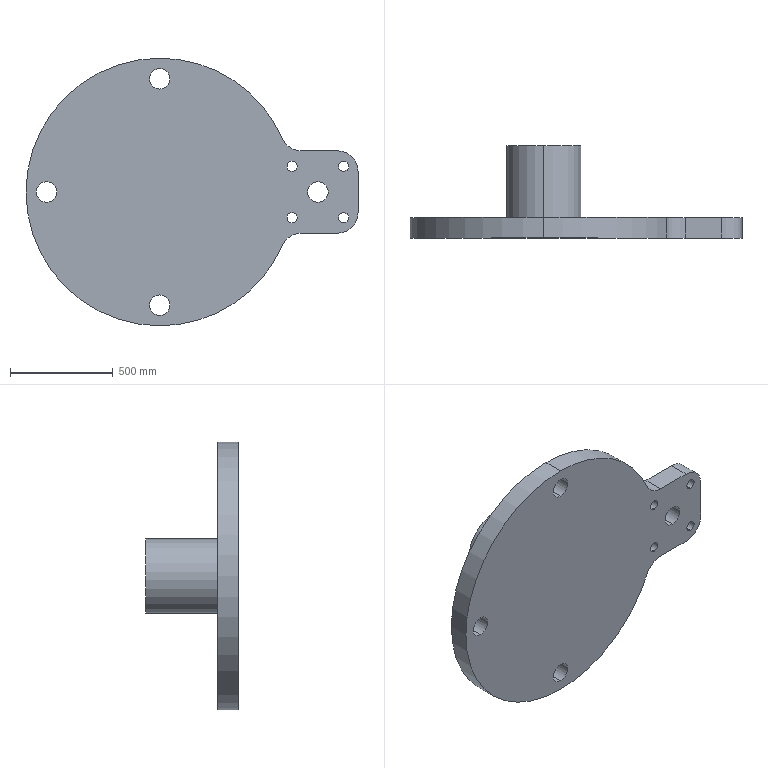Part | SolidWorks | features ICE 9, Extrusion 1, Fillet 1, MirrorPattern 1 | 1 solid | 31 faces | box 1613 x 450 x 1300 mm | volume 177120660 mm3 | cylinder 25 | plane 6 | commonest cylinder face diameters 50 x8 100 x8 200 x4 1300 x3 360 x2
STEP:
#1=CARTESIAN_POINT('',(768.466,750.,50.));
#2=VERTEX_POINT('',#1);
#3=CARTESIAN_POINT('',(768.466,750.,-50.));
#4=VERTEX_POINT('',#3);
#5=CARTESIAN_POINT('',(768.466,750.,0.));
#6=DIRECTION('',(0.,-1.,0.));
#7=DIRECTION('',(0.,0.,1.));
#8=AXIS2_PLACEMENT_3D('',#5,#6,#7);
#9=CIRCLE('',#8,50.);
#10=EDGE_CURVE('',#2,#4,#9,.T.);
#11=ORIENTED_EDGE('',*,*,#10,.T.);
#12=CARTESIAN_POINT('',(768.466,850.,-50.));
#13=VERTEX_POINT('',#12);
#14=CARTESIAN_POINT('',(768.466,-1050.001,-50.));
#15=DIRECTION('',(0.,1.,0.));
#16=VECTOR('',#15,1000.);
#17=LINE('',#14,#16);
#18=EDGE_CURVE('',#4,#13,#17,.T.);
#19=ORIENTED_EDGE('',*,*,#18,.T.);
#20=CARTESIAN_POINT('',(768.466,850.,50.));
#21=VERTEX_POINT('',#20);
#22=CARTESIAN_POINT('',(768.466,850.,0.));
#23=DIRECTION('',(0.,1.,0.));
#24=DIRECTION('',(0.,0.,1.));
#25=AXIS2_PLACEMENT_3D('',#22,#23,#24);
#26=CIRCLE('',#25,50.);
#27=EDGE_CURVE('',#13,#21,#26,.T.);
#28=ORIENTED_EDGE('',*,*,#27,.T.);
#29=CARTESIAN_POINT('',(768.466,-1050.001,50.));
#30=DIRECTION('',(0.,1.,0.));
#31=VECTOR('',#30,1000.);
#32=LINE('',#29,#31);
#33=EDGE_CURVE('',#2,#21,#32,.T.);
#34=ORIENTED_EDGE('',*,*,#33,.F.);
#35=EDGE_LOOP('',(#11,#19,#28,#34));
#36=FACE_OUTER_BOUND('',#35,.T.);
#37=CARTESIAN_POINT('',(768.466,-1050.001,0.));
#38=DIRECTION('',(0.,1.,0.));
#39=DIRECTION('',(0.,0.,1.));
#40=AXIS2_PLACEMENT_3D('',#37,#38,#39);
#41=CYLINDRICAL_SURFACE('',#40,50.);
#42=ADVANCED_FACE('',(#36),#41,.F.);
#43=CARTESIAN_POINT('',(893.466,750.,150.));
#44=VERTEX_POINT('',#43);
#45=CARTESIAN_POINT('',(893.466,750.,100.));
#46=VERTEX_POINT('',#45);
#47=CARTESIAN_POINT('',(893.466,750.,125.));
#48=DIRECTION('',(0.,-1.,0.));
#49=DIRECTION('',(0.,0.,1.));
#50=AXIS2_PLACEMENT_3D('',#47,#48,#49);
#51=CIRCLE('',#50,25.);
#52=EDGE_CURVE('',#44,#46,#51,.T.);
#53=ORIENTED_EDGE('',*,*,#52,.T.);
#54=CARTESIAN_POINT('',(893.466,850.,100.));
#55=VERTEX_POINT('',#54);
#56=CARTESIAN_POINT('',(893.466,-1050.001,100.));
#57=DIRECTION('',(0.,1.,0.));
#58=VECTOR('',#57,1000.);
#59=LINE('',#56,#58);
#60=EDGE_CURVE('',#46,#55,#59,.T.);
#61=ORIENTED_EDGE('',*,*,#60,.T.);
#62=CARTESIAN_POINT('',(893.466,850.,150.));
#63=VERTEX_POINT('',#62);
#64=CARTESIAN_POINT('',(893.466,850.,125.));
#65=DIRECTION('',(0.,1.,0.));
#66=DIRECTION('',(0.,0.,1.));
#67=AXIS2_PLACEMENT_3D('',#64,#65,#66);
#68=CIRCLE('',#67,25.);
#69=EDGE_CURVE('',#55,#63,#68,.T.);
#70=ORIENTED_EDGE('',*,*,#69,.T.);
#71=CARTESIAN_POINT('',(893.466,-1050.001,150.));
#72=DIRECTION('',(0.,1.,0.));
#73=VECTOR('',#72,1000.);
#74=LINE('',#71,#73);
#75=EDGE_CURVE('',#44,#63,#74,.T.);
#76=ORIENTED_EDGE('',*,*,#75,.F.);
#77=EDGE_LOOP('',(#53,#61,#70,#76));
#78=FACE_OUTER_BOUND('',#77,.T.);
#79=CARTESIAN_POINT('',(893.466,-1050.001,125.));
#80=DIRECTION('',(0.,1.,0.));
#81=DIRECTION('',(0.,0.,1.));
#82=AXIS2_PLACEMENT_3D('',#79,#80,#81);
#83=CYLINDRICAL_SURFACE('',#82,25.);
#84=ADVANCED_FACE('',(#78),#83,.F.);
#85=CARTESIAN_POINT('',(643.466,750.,150.));
#86=VERTEX_POINT('',#85);
#87=CARTESIAN_POINT('',(643.466,750.,100.));
#88=VERTEX_POINT('',#87);
#89=CARTESIAN_POINT('',(643.466,750.,125.));
#90=DIRECTION('',(0.,-1.,0.));
#91=DIRECTION('',(0.,0.,1.));
#92=AXIS2_PLACEMENT_3D('',#89,#90,#91);
#93=CIRCLE('',#92,25.);
#94=EDGE_CURVE('',#86,#88,#93,.T.);
#95=ORIENTED_EDGE('',*,*,#94,.T.);
#96=CARTESIAN_POINT('',(643.466,850.,100.));
#97=VERTEX_POINT('',#96);
#98=CARTESIAN_POINT('',(643.466,-1050.001,100.));
#99=DIRECTION('',(0.,1.,0.));
#100=VECTOR('',#99,1000.);
#101=LINE('',#98,#100);
#102=EDGE_CURVE('',#88,#97,#101,.T.);
#103=ORIENTED_EDGE('',*,*,#102,.T.);
#104=CARTESIAN_POINT('',(643.466,850.,150.));
#105=VERTEX_POINT('',#104);
#106=CARTESIAN_POINT('',(643.466,850.,125.));
#107=DIRECTION('',(0.,1.,0.));
#108=DIRECTION('',(0.,0.,1.));
#109=AXIS2_PLACEMENT_3D('',#106,#107,#108);
#110=CIRCLE('',#109,25.);
#111=EDGE_CURVE('',#97,#105,#110,.T.);
#112=ORIENTED_EDGE('',*,*,#111,.T.);
#113=CARTESIAN_POINT('',(643.466,-1050.001,150.));
#114=DIRECTION('',(0.,1.,0.));
#115=VECTOR('',#114,1000.);
#116=LINE('',#113,#115);
#117=EDGE_CURVE('',#86,#105,#116,.T.);
#118=ORIENTED_EDGE('',*,*,#117,.F.);
#119=EDGE_LOOP('',(#95,#103,#112,#118));
#120=FACE_OUTER_BOUND('',#119,.T.);
#121=CARTESIAN_POINT('',(643.466,-1050.001,125.));
#122=DIRECTION('',(0.,1.,0.));
#123=DIRECTION('',(0.,0.,1.));
#124=AXIS2_PLACEMENT_3D('',#121,#122,#123);
#125=CYLINDRICAL_SURFACE('',#124,25.);
#126=ADVANCED_FACE('',(#120),#125,.F.);
#127=CARTESIAN_POINT('',(643.466,750.,-100.));
#128=VERTEX_POINT('',#127);
#129=CARTESIAN_POINT('',(643.466,750.,-150.));
#130=VERTEX_POINT('',#129);
#131=CARTESIAN_POINT('',(643.466,750.,-125.));
#132=DIRECTION('',(0.,-1.,0.));
#133=DIRECTION('',(0.,0.,1.));
#134=AXIS2_PLACEMENT_3D('',#131,#132,#133);
#135=CIRCLE('',#134,25.);
#136=EDGE_CURVE('',#128,#130,#135,.T.);
#137=ORIENTED_EDGE('',*,*,#136,.T.);
#138=CARTESIAN_POINT('',(643.466,850.,-150.));
#139=VERTEX_POINT('',#138);
#140=CARTESIAN_POINT('',(643.466,-1050.001,-150.));
#141=DIRECTION('',(0.,1.,0.));
#142=VECTOR('',#141,1000.);
#143=LINE('',#140,#142);
#144=EDGE_CURVE('',#130,#139,#143,.T.);
#145=ORIENTED_EDGE('',*,*,#144,.T.);
#146=CARTESIAN_POINT('',(643.466,850.,-100.));
#147=VERTEX_POINT('',#146);
#148=CARTESIAN_POINT('',(643.466,850.,-125.));
#149=DIRECTION('',(0.,1.,0.));
#150=DIRECTION('',(0.,0.,1.));
#151=AXIS2_PLACEMENT_3D('',#148,#149,#150);
#152=CIRCLE('',#151,25.);
#153=EDGE_CURVE('',#139,#147,#152,.T.);
#154=ORIENTED_EDGE('',*,*,#153,.T.);
#155=CARTESIAN_POINT('',(643.466,-1050.001,-100.));
#156=DIRECTION('',(0.,1.,0.));
#157=VECTOR('',#156,1000.);
#158=LINE('',#155,#157);
#159=EDGE_CURVE('',#128,#147,#158,.T.);
#160=ORIENTED_EDGE('',*,*,#159,.F.);
#161=EDGE_LOOP('',(#137,#145,#154,#160));
#162=FACE_OUTER_BOUND('',#161,.T.);
#163=CARTESIAN_POINT('',(643.466,-1050.001,-125.));
#164=DIRECTION('',(0.,1.,0.));
#165=DIRECTION('',(0.,0.,1.));
#166=AXIS2_PLACEMENT_3D('',#163,#164,#165);
#167=CYLINDRICAL_SURFACE('',#166,25.);
#168=ADVANCED_FACE('',(#162),#167,.F.);
#169=CARTESIAN_POINT('',(893.466,750.,-100.));
#170=VERTEX_POINT('',#169);
#171=CARTESIAN_POINT('',(893.466,750.,-150.));
#172=VERTEX_POINT('',#171);
#173=CARTESIAN_POINT('',(893.466,750.,-125.));
#174=DIRECTION('',(0.,-1.,0.));
#175=DIRECTION('',(0.,0.,1.));
#176=AXIS2_PLACEMENT_3D('',#173,#174,#175);
#177=CIRCLE('',#176,25.);
#178=EDGE_CURVE('',#170,#172,#177,.T.);
#179=ORIENTED_EDGE('',*,*,#178,.T.);
#180=CARTESIAN_POINT('',(893.466,850.,-150.));
#181=VERTEX_POINT('',#180);
#182=CARTESIAN_POINT('',(893.466,-1050.001,-150.));
#183=DIRECTION('',(0.,1.,0.));
#184=VECTOR('',#183,1000.);
#185=LINE('',#182,#184);
#186=EDGE_CURVE('',#172,#181,#185,.T.);
#187=ORIENTED_EDGE('',*,*,#186,.T.);
#188=CARTESIAN_POINT('',(893.466,850.,-100.));
#189=VERTEX_POINT('',#188);
#190=CARTESIAN_POINT('',(893.466,850.,-125.));
#191=DIRECTION('',(0.,1.,0.));
#192=DIRECTION('',(0.,0.,1.));
#193=AXIS2_PLACEMENT_3D('',#190,#191,#192);
#194=CIRCLE('',#193,25.);
#195=EDGE_CURVE('',#181,#189,#194,.T.);
#196=ORIENTED_EDGE('',*,*,#195,.T.);
#197=CARTESIAN_POINT('',(893.466,-1050.001,-100.));
#198=DIRECTION('',(0.,1.,0.));
#199=VECTOR('',#198,1000.);
#200=LINE('',#197,#199);
#201=EDGE_CURVE('',#170,#189,#200,.T.);
#202=ORIENTED_EDGE('',*,*,#201,.F.);
#203=EDGE_LOOP('',(#179,#187,#196,#202));
#204=FACE_OUTER_BOUND('',#203,.T.);
#205=CARTESIAN_POINT('',(893.466,-1050.001,-125.));
#206=DIRECTION('',(0.,1.,0.));
#207=DIRECTION('',(0.,0.,1.));
#208=AXIS2_PLACEMENT_3D('',#205,#206,#207);
#209=CYLINDRICAL_SURFACE('',#208,25.);
#210=ADVANCED_FACE('',(#204),#209,.F.);
#211=CARTESIAN_POINT('',(0.,1200.,180.));
#212=VERTEX_POINT('',#211);
#213=CARTESIAN_POINT('',(0.,1200.,-180.));
#214=VERTEX_POINT('',#213);
#215=CARTESIAN_POINT('',(0.,1200.,0.));
#216=DIRECTION('',(0.,1.,0.));
#217=DIRECTION('',(0.,0.,1.));
#218=AXIS2_PLACEMENT_3D('',#215,#216,#217);
#219=CIRCLE('',#218,180.);
#220=EDGE_CURVE('',#212,#214,#219,.T.);
#221=ORIENTED_EDGE('',*,*,#220,.F.);
#222=CARTESIAN_POINT('',(0.,850.,180.));
#223=VERTEX_POINT('',#222);
#224=CARTESIAN_POINT('',(0.,1200.,180.));
#225=DIRECTION('',(0.,-1.,0.));
#226=VECTOR('',#225,1000.);
#227=LINE('',#224,#226);
#228=EDGE_CURVE('',#212,#223,#227,.T.);
#229=ORIENTED_EDGE('',*,*,#228,.T.);
#230=CARTESIAN_POINT('',(0.,850.,-180.));
#231=VERTEX_POINT('',#230);
#232=CARTESIAN_POINT('',(0.,850.,0.));
#233=DIRECTION('',(0.,1.,0.));
#234=DIRECTION('',(0.,0.,1.));
#235=AXIS2_PLACEMENT_3D('',#232,#233,#234);
#236=CIRCLE('',#235,180.);
#237=EDGE_CURVE('',#223,#231,#236,.T.);
#238=ORIENTED_EDGE('',*,*,#237,.T.);
#239=CARTESIAN_POINT('',(0.,1200.,-180.));
#240=DIRECTION('',(0.,-1.,0.));
#241=VECTOR('',#240,1000.);
#242=LINE('',#239,#241);
#243=EDGE_CURVE('',#214,#231,#242,.T.);
#244=ORIENTED_EDGE('',*,*,#243,.F.);
#245=EDGE_LOOP('',(#221,#229,#238,#244));
#246=FACE_OUTER_BOUND('',#245,.T.);
#247=CARTESIAN_POINT('',(0.,1200.,0.));
#248=DIRECTION('',(0.,-1.,0.));
#249=DIRECTION('',(0.,0.,-1.));
#250=AXIS2_PLACEMENT_3D('',#247,#248,#249);
#251=CYLINDRICAL_SURFACE('',#250,180.);
#252=ADVANCED_FACE('',(#246),#251,.T.);
#253=CARTESIAN_POINT('',(0.,750.,600.));
#254=VERTEX_POINT('',#253);
#255=CARTESIAN_POINT('',(0.,750.,500.));
#256=VERTEX_POINT('',#255);
#257=CARTESIAN_POINT('',(0.,750.,550.));
#258=DIRECTION('',(0.,-1.,0.));
#259=DIRECTION('',(0.,0.,1.));
#260=AXIS2_PLACEMENT_3D('',#257,#258,#259);
#261=CIRCLE('',#260,50.);
#262=EDGE_CURVE('',#254,#256,#261,.T.);
#263=ORIENTED_EDGE('',*,*,#262,.T.);
#264=CARTESIAN_POINT('',(0.,850.,500.));
#265=VERTEX_POINT('',#264);
#266=CARTESIAN_POINT('',(0.,-1050.,500.));
#267=DIRECTION('',(0.,1.,0.));
#268=VECTOR('',#267,1000.);
#269=LINE('',#266,#268);
#270=EDGE_CURVE('',#256,#265,#269,.T.);
#271=ORIENTED_EDGE('',*,*,#270,.T.);
#272=CARTESIAN_POINT('',(0.,850.,600.));
#273=VERTEX_POINT('',#272);
#274=CARTESIAN_POINT('',(0.,850.,550.));
#275=DIRECTION('',(0.,-1.,0.));
#276=DIRECTION('',(0.,0.,-1.));
#277=AXIS2_PLACEMENT_3D('',#274,#275,#276);
#278=CIRCLE('',#277,50.);
#279=EDGE_CURVE('',#273,#265,#278,.T.);
#280=ORIENTED_EDGE('',*,*,#279,.F.);
#281=CARTESIAN_POINT('',(0.,-1050.,600.));
#282=DIRECTION('',(0.,1.,0.));
#283=VECTOR('',#282,1000.);
#284=LINE('',#281,#283);
#285=EDGE_CURVE('',#254,#273,#284,.T.);
#286=ORIENTED_EDGE('',*,*,#285,.F.);
#287=EDGE_LOOP('',(#263,#271,#280,#286));
#288=FACE_OUTER_BOUND('',#287,.T.);
#289=CARTESIAN_POINT('',(0.,-1050.,550.));
#290=DIRECTION('',(0.,1.,0.));
#291=DIRECTION('',(0.,0.,1.));
#292=AXIS2_PLACEMENT_3D('',#289,#290,#291);
#293=CYLINDRICAL_SURFACE('',#292,50.);
#294=ADVANCED_FACE('',(#288),#293,.F.);
#295=CARTESIAN_POINT('',(0.,750.,-500.));
#296=VERTEX_POINT('',#295);
#297=CARTESIAN_POINT('',(0.,750.,-600.));
#298=VERTEX_POINT('',#297);
#299=CARTESIAN_POINT('',(0.,750.,-550.));
#300=DIRECTION('',(0.,-1.,0.));
#301=DIRECTION('',(0.,0.,1.));
#302=AXIS2_PLACEMENT_3D('',#299,#300,#301);
#303=CIRCLE('',#302,50.);
#304=EDGE_CURVE('',#296,#298,#303,.T.);
#305=ORIENTED_EDGE('',*,*,#304,.T.);
#306=CARTESIAN_POINT('',(0.,850.,-600.));
#307=VERTEX_POINT('',#306);
#308=CARTESIAN_POINT('',(0.,-1050.,-600.));
#309=DIRECTION('',(0.,1.,0.));
#310=VECTOR('',#309,1000.);
#311=LINE('',#308,#310);
#312=EDGE_CURVE('',#298,#307,#311,.T.);
#313=ORIENTED_EDGE('',*,*,#312,.T.);
#314=CARTESIAN_POINT('',(0.,850.,-500.));
#315=VERTEX_POINT('',#314);
#316=CARTESIAN_POINT('',(0.,850.,-550.));
#317=DIRECTION('',(0.,-1.,0.));
#318=DIRECTION('',(0.,0.,-1.));
#319=AXIS2_PLACEMENT_3D('',#316,#317,#318);
#320=CIRCLE('',#319,50.);
#321=EDGE_CURVE('',#315,#307,#320,.T.);
#322=ORIENTED_EDGE('',*,*,#321,.F.);
#323=CARTESIAN_POINT('',(0.,-1050.,-500.));
#324=DIRECTION('',(0.,1.,0.));
#325=VECTOR('',#324,1000.);
#326=LINE('',#323,#325);
#327=EDGE_CURVE('',#296,#315,#326,.T.);
#328=ORIENTED_EDGE('',*,*,#327,.F.);
#329=EDGE_LOOP('',(#305,#313,#322,#328));
#330=FACE_OUTER_BOUND('',#329,.T.);
#331=CARTESIAN_POINT('',(0.,-1050.,-550.));
#332=DIRECTION('',(0.,1.,0.));
#333=DIRECTION('',(0.,0.,1.));
#334=AXIS2_PLACEMENT_3D('',#331,#332,#333);
#335=CYLINDRICAL_SURFACE('',#334,50.);
#336=ADVANCED_FACE('',(#330),#335,.F.);
#337=CARTESIAN_POINT('',(-550.,750.,50.));
#338=VERTEX_POINT('',#337);
#339=CARTESIAN_POINT('',(-550.,750.,-50.));
#340=VERTEX_POINT('',#339);
#341=CARTESIAN_POINT('',(-550.,750.,0.));
#342=DIRECTION('',(0.,-1.,0.));
#343=DIRECTION('',(0.,0.,1.));
#344=AXIS2_PLACEMENT_3D('',#341,#342,#343);
#345=CIRCLE('',#344,50.);
#346=EDGE_CURVE('',#338,#340,#345,.T.);
#347=ORIENTED_EDGE('',*,*,#346,.T.);
#348=CARTESIAN_POINT('',(-550.,850.,-50.));
#349=VERTEX_POINT('',#348);
#350=CARTESIAN_POINT('',(-550.,-1050.,-50.));
#351=DIRECTION('',(0.,1.,0.));
#352=VECTOR('',#351,1000.);
#353=LINE('',#350,#352);
#354=EDGE_CURVE('',#340,#349,#353,.T.);
#355=ORIENTED_EDGE('',*,*,#354,.T.);
#356=CARTESIAN_POINT('',(-550.,850.,50.));
#357=VERTEX_POINT('',#356);
#358=CARTESIAN_POINT('',(-550.,850.,0.));
#359=DIRECTION('',(0.,-1.,0.));
#360=DIRECTION('',(0.,0.,-1.));
#361=AXIS2_PLACEMENT_3D('',#358,#359,#360);
#362=CIRCLE('',#361,50.);
#363=EDGE_CURVE('',#357,#349,#362,.T.);
#364=ORIENTED_EDGE('',*,*,#363,.F.);
#365=CARTESIAN_POINT('',(-550.,-1050.,50.));
#366=DIRECTION('',(0.,1.,0.));
#367=VECTOR('',#366,1000.);
#368=LINE('',#365,#367);
#369=EDGE_CURVE('',#338,#357,#368,.T.);
#370=ORIENTED_EDGE('',*,*,#369,.F.);
#371=EDGE_LOOP('',(#347,#355,#364,#370));
#372=FACE_OUTER_BOUND('',#371,.T.);
#373=CARTESIAN_POINT('',(-550.,-1050.,0.));
#374=DIRECTION('',(0.,1.,0.));
#375=DIRECTION('',(0.,0.,1.));
#376=AXIS2_PLACEMENT_3D('',#373,#374,#375);
#377=CYLINDRICAL_SURFACE('',#376,50.);
#378=ADVANCED_FACE('',(#372),#377,.F.);
#379=CARTESIAN_POINT('',(595.735,850.,260.));
#380=VERTEX_POINT('',#379);
#381=CARTESIAN_POINT('',(0.,850.,650.));
#382=VERTEX_POINT('',#381);
#383=CARTESIAN_POINT('',(0.,850.,0.));
#384=DIRECTION('',(0.,-1.,0.));
#385=DIRECTION('',(0.,0.,-1.));
#386=AXIS2_PLACEMENT_3D('',#383,#384,#385);
#387=CIRCLE('',#386,650.);
#388=EDGE_CURVE('',#380,#382,#387,.T.);
#389=ORIENTED_EDGE('',*,*,#388,.T.);
#390=CARTESIAN_POINT('',(0.,750.,650.));
#391=VERTEX_POINT('',#390);
#392=CARTESIAN_POINT('',(0.,850.,650.));
#393=DIRECTION('',(0.,-1.,0.));
#394=VECTOR('',#393,1000.);
#395=LINE('',#392,#394);
#396=EDGE_CURVE('',#382,#391,#395,.T.);
#397=ORIENTED_EDGE('',*,*,#396,.T.);
#398=CARTESIAN_POINT('',(595.735,750.,260.));
#399=VERTEX_POINT('',#398);
#400=CARTESIAN_POINT('',(0.,750.,0.));
#401=DIRECTION('',(0.,-1.,0.));
#402=DIRECTION('',(0.,0.,-1.));
#403=AXIS2_PLACEMENT_3D('',#400,#401,#402);
#404=CIRCLE('',#403,650.);
#405=EDGE_CURVE('',#399,#391,#404,.T.);
#406=ORIENTED_EDGE('',*,*,#405,.F.);
#407=CARTESIAN_POINT('',(595.735,850.,260.));
#408=DIRECTION('',(0.,1.,0.));
#409=VECTOR('',#408,1000.);
#410=LINE('',#407,#409);
#411=EDGE_CURVE('',#399,#380,#410,.T.);
#412=ORIENTED_EDGE('',*,*,#411,.T.);
#413=EDGE_LOOP('',(#389,#397,#406,#412));
#414=FACE_OUTER_BOUND('',#413,.T.);
#415=CARTESIAN_POINT('',(0.,850.,0.));
#416=DIRECTION('',(0.,-1.,0.));
#417=DIRECTION('',(0.,0.,-1.));
#418=AXIS2_PLACEMENT_3D('',#415,#416,#417);
#419=CYLINDRICAL_SURFACE('',#418,650.);
#420=ADVANCED_FACE('',(#414),#419,.T.);
#421=ORIENTED_EDGE('',*,*,#396,.F.);
#422=CARTESIAN_POINT('',(0.,850.,-650.));
#423=VERTEX_POINT('',#422);
#424=CARTESIAN_POINT('',(0.,850.,0.));
#425=DIRECTION('',(0.,-1.,0.));
#426=DIRECTION('',(0.,0.,-1.));
#427=AXIS2_PLACEMENT_3D('',#424,#425,#426);
#428=CIRCLE('',#427,650.);
#429=EDGE_CURVE('',#382,#423,#428,.T.);
#430=ORIENTED_EDGE('',*,*,#429,.T.);
#431=CARTESIAN_POINT('',(0.,750.,-650.));
#432=VERTEX_POINT('',#431);
#433=CARTESIAN_POINT('',(0.,850.,-650.));
#434=DIRECTION('',(0.,-1.,0.));
#435=VECTOR('',#434,1000.);
#436=LINE('',#433,#435);
#437=EDGE_CURVE('',#423,#432,#436,.T.);
#438=ORIENTED_EDGE('',*,*,#437,.T.);
#439=CARTESIAN_POINT('',(0.,750.,0.));
#440=DIRECTION('',(0.,-1.,0.));
#441=DIRECTION('',(0.,0.,-1.));
#442=AXIS2_PLACEMENT_3D('',#439,#440,#441);
#443=CIRCLE('',#442,650.);
#444=EDGE_CURVE('',#391,#432,#443,.T.);
#445=ORIENTED_EDGE('',*,*,#444,.F.);
#446=EDGE_LOOP('',(#421,#430,#438,#445));
#447=FACE_OUTER_BOUND('',#446,.T.);
#448=CARTESIAN_POINT('',(0.,850.,0.));
#449=DIRECTION('',(0.,-1.,0.));
#450=DIRECTION('',(0.,0.,-1.));
#451=AXIS2_PLACEMENT_3D('',#448,#449,#450);
#452=CYLINDRICAL_SURFACE('',#451,650.);
#453=ADVANCED_FACE('',(#447),#452,.T.);
#454=ORIENTED_EDGE('',*,*,#437,.F.);
#455=CARTESIAN_POINT('',(595.735,850.,-260.));
#456=VERTEX_POINT('',#455);
#457=CARTESIAN_POINT('',(0.,850.,0.));
#458=DIRECTION('',(0.,-1.,0.));
#459=DIRECTION('',(0.,0.,-1.));
#460=AXIS2_PLACEMENT_3D('',#457,#458,#459);
#461=CIRCLE('',#460,650.);
#462=EDGE_CURVE('',#423,#456,#461,.T.);
#463=ORIENTED_EDGE('',*,*,#462,.T.);
#464=CARTESIAN_POINT('',(595.735,750.,-260.));
#465=VERTEX_POINT('',#464);
#466=CARTESIAN_POINT('',(595.735,850.,-260.));
#467=DIRECTION('',(0.,-1.,0.));
#468=VECTOR('',#467,1000.);
#469=LINE('',#466,#468);
#470=EDGE_CURVE('',#456,#465,#469,.T.);
#471=ORIENTED_EDGE('',*,*,#470,.T.);
#472=CARTESIAN_POINT('',(0.,750.,0.));
#473=DIRECTION('',(0.,-1.,0.));
#474=DIRECTION('',(0.,0.,-1.));
#475=AXIS2_PLACEMENT_3D('',#472,#473,#474);
#476=CIRCLE('',#475,650.);
#477=EDGE_CURVE('',#432,#465,#476,.T.);
#478=ORIENTED_EDGE('',*,*,#477,.F.);
#479=EDGE_LOOP('',(#454,#463,#471,#478));
#480=FACE_OUTER_BOUND('',#479,.T.);
#481=CARTESIAN_POINT('',(0.,850.,0.));
#482=DIRECTION('',(0.,-1.,0.));
#483=DIRECTION('',(0.,0.,-1.));
#484=AXIS2_PLACEMENT_3D('',#481,#482,#483);
#485=CYLINDRICAL_SURFACE('',#484,650.);
#486=ADVANCED_FACE('',(#480),#485,.T.);
#487=CARTESIAN_POINT('',(768.466,850.,0.));
#488=DIRECTION('',(0.,1.,0.));
#489=DIRECTION('',(0.,0.,1.));
#490=AXIS2_PLACEMENT_3D('',#487,#488,#489);
#491=CIRCLE('',#490,50.);
#492=EDGE_CURVE('',#21,#13,#491,.T.);
#493=ORIENTED_EDGE('',*,*,#492,.F.);
#494=ORIENTED_EDGE('',*,*,#27,.F.);
#495=EDGE_LOOP('',(#493,#494));
#496=FACE_BOUND('',#495,.T.);
#497=CARTESIAN_POINT('',(893.466,850.,125.));
#498=DIRECTION('',(0.,1.,0.));
#499=DIRECTION('',(0.,0.,1.));
#500=AXIS2_PLACEMENT_3D('',#497,#498,#499);
#501=CIRCLE('',#500,25.);
#502=EDGE_CURVE('',#63,#55,#501,.T.);
#503=ORIENTED_EDGE('',*,*,#502,.F.);
#504=ORIENTED_EDGE('',*,*,#69,.F.);
#505=EDGE_LOOP('',(#503,#504));
#506=FACE_BOUND('',#505,.T.);
#507=CARTESIAN_POINT('',(643.466,850.,125.));
#508=DIRECTION('',(0.,1.,0.));
#509=DIRECTION('',(0.,0.,1.));
#510=AXIS2_PLACEMENT_3D('',#507,#508,#509);
#511=CIRCLE('',#510,25.);
#512=EDGE_CURVE('',#105,#97,#511,.T.);
#513=ORIENTED_EDGE('',*,*,#512,.F.);
#514=ORIENTED_EDGE('',*,*,#111,.F.);
#515=EDGE_LOOP('',(#513,#514));
#516=FACE_BOUND('',#515,.T.);
#517=CARTESIAN_POINT('',(643.466,850.,-125.));
#518=DIRECTION('',(0.,1.,0.));
#519=DIRECTION('',(0.,0.,1.));
#520=AXIS2_PLACEMENT_3D('',#517,#518,#519);
#521=CIRCLE('',#520,25.);
#522=EDGE_CURVE('',#147,#139,#521,.T.);
#523=ORIENTED_EDGE('',*,*,#522,.F.);
#524=ORIENTED_EDGE('',*,*,#153,.F.);
#525=EDGE_LOOP('',(#523,#524));
#526=FACE_BOUND('',#525,.T.);
#527=CARTESIAN_POINT('',(893.466,850.,-125.));
#528=DIRECTION('',(0.,1.,0.));
#529=DIRECTION('',(0.,0.,1.));
#530=AXIS2_PLACEMENT_3D('',#527,#528,#529);
#531=CIRCLE('',#530,25.);
#532=EDGE_CURVE('',#189,#181,#531,.T.);
#533=ORIENTED_EDGE('',*,*,#532,.F.);
#534=ORIENTED_EDGE('',*,*,#195,.F.);
#535=EDGE_LOOP('',(#533,#534));
#536=FACE_BOUND('',#535,.T.);
#537=CARTESIAN_POINT('',(687.386,850.,200.));
#538=VERTEX_POINT('',#537);
#539=CARTESIAN_POINT('',(863.466,850.,200.));
#540=VERTEX_POINT('',#539);
#541=CARTESIAN_POINT('',(618.466,850.,200.));
#542=DIRECTION('',(1.,0.,0.));
#543=VECTOR('',#542,1000.);
#544=LINE('',#541,#543);
#545=EDGE_CURVE('',#538,#540,#544,.T.);
#546=ORIENTED_EDGE('',*,*,#545,.T.);
#547=CARTESIAN_POINT('',(963.466,850.,100.));
#548=VERTEX_POINT('',#547);
#549=CARTESIAN_POINT('',(863.466,850.,100.));
#550=DIRECTION('',(0.,1.,0.));
#551=DIRECTION('',(0.,0.,1.));
#552=AXIS2_PLACEMENT_3D('',#549,#550,#551);
#553=CIRCLE('',#552,100.);
#554=EDGE_CURVE('',#540,#548,#553,.T.);
#555=ORIENTED_EDGE('',*,*,#554,.T.);
#556=CARTESIAN_POINT('',(963.466,850.,-100.));
#557=VERTEX_POINT('',#556);
#558=CARTESIAN_POINT('',(963.466,850.,-200.));
#559=DIRECTION('',(0.,0.,-1.));
#560=VECTOR('',#559,1000.);
#561=LINE('',#558,#560);
#562=EDGE_CURVE('',#548,#557,#561,.T.);
#563=ORIENTED_EDGE('',*,*,#562,.T.);
#564=CARTESIAN_POINT('',(863.466,850.,-200.));
#565=VERTEX_POINT('',#564);
#566=CARTESIAN_POINT('',(863.466,850.,-100.));
#567=DIRECTION('',(0.,1.,0.));
#568=DIRECTION('',(0.,0.,1.));
#569=AXIS2_PLACEMENT_3D('',#566,#567,#568);
#570=CIRCLE('',#569,100.);
#571=EDGE_CURVE('',#557,#565,#570,.T.);
#572=ORIENTED_EDGE('',*,*,#571,.T.);
#573=CARTESIAN_POINT('',(687.386,850.,-200.));
#574=VERTEX_POINT('',#573);
#575=CARTESIAN_POINT('',(618.466,850.,-200.));
#576=DIRECTION('',(-1.,0.,0.));
#577=VECTOR('',#576,1000.);
#578=LINE('',#575,#577);
#579=EDGE_CURVE('',#565,#574,#578,.T.);
#580=ORIENTED_EDGE('',*,*,#579,.T.);
#581=CARTESIAN_POINT('',(687.386,850.,-300.));
#582=DIRECTION('',(0.,-1.,0.));
#583=DIRECTION('',(0.,0.,1.));
#584=AXIS2_PLACEMENT_3D('',#581,#582,#583);
#585=CIRCLE('',#584,100.);
#586=EDGE_CURVE('',#574,#456,#585,.T.);
#587=ORIENTED_EDGE('',*,*,#586,.T.);
#588=ORIENTED_EDGE('',*,*,#462,.F.);
#589=ORIENTED_EDGE('',*,*,#429,.F.);
#590=ORIENTED_EDGE('',*,*,#388,.F.);
#591=CARTESIAN_POINT('',(687.386,850.,300.));
#592=DIRECTION('',(0.,-1.,0.));
#593=DIRECTION('',(0.,0.,1.));
#594=AXIS2_PLACEMENT_3D('',#591,#592,#593);
#595=CIRCLE('',#594,100.);
#596=EDGE_CURVE('',#380,#538,#595,.T.);
#597=ORIENTED_EDGE('',*,*,#596,.T.);
#598=EDGE_LOOP('',(#546,#555,#563,#572,#580,#587,#588,#589,#590,#597));
#599=FACE_OUTER_BOUND('',#598,.T.);
#600=CARTESIAN_POINT('',(0.,850.,0.));
#601=DIRECTION('',(0.,1.,0.));
#602=DIRECTION('',(0.,0.,1.));
#603=AXIS2_PLACEMENT_3D('',#600,#601,#602);
#604=CIRCLE('',#603,180.);
#605=EDGE_CURVE('',#231,#223,#604,.T.);
#606=ORIENTED_EDGE('',*,*,#605,.F.);
#607=ORIENTED_EDGE('',*,*,#237,.F.);
#608=EDGE_LOOP('',(#606,#607));
#609=FACE_BOUND('',#608,.T.);
#610=ORIENTED_EDGE('',*,*,#279,.T.);
#611=CARTESIAN_POINT('',(0.,850.,550.));
#612=DIRECTION('',(0.,-1.,0.));
#613=DIRECTION('',(0.,0.,-1.));
#614=AXIS2_PLACEMENT_3D('',#611,#612,#613);
#615=CIRCLE('',#614,50.);
#616=EDGE_CURVE('',#265,#273,#615,.T.);
#617=ORIENTED_EDGE('',*,*,#616,.T.);
#618=EDGE_LOOP('',(#610,#617));
#619=FACE_BOUND('',#618,.T.);
#620=ORIENTED_EDGE('',*,*,#321,.T.);
#621=CARTESIAN_POINT('',(0.,850.,-550.));
#622=DIRECTION('',(0.,-1.,0.));
#623=DIRECTION('',(0.,0.,-1.));
#624=AXIS2_PLACEMENT_3D('',#621,#622,#623);
#625=CIRCLE('',#624,50.);
#626=EDGE_CURVE('',#307,#315,#625,.T.);
#627=ORIENTED_EDGE('',*,*,#626,.T.);
#628=EDGE_LOOP('',(#620,#627));
#629=FACE_BOUND('',#628,.T.);
#630=ORIENTED_EDGE('',*,*,#363,.T.);
#631=CARTESIAN_POINT('',(-550.,850.,0.));
#632=DIRECTION('',(0.,-1.,0.));
#633=DIRECTION('',(0.,0.,-1.));
#634=AXIS2_PLACEMENT_3D('',#631,#632,#633);
#635=CIRCLE('',#634,50.);
#636=EDGE_CURVE('',#349,#357,#635,.T.);
#637=ORIENTED_EDGE('',*,*,#636,.T.);
#638=EDGE_LOOP('',(#630,#637));
#639=FACE_BOUND('',#638,.T.);
#640=CARTESIAN_POINT('',(0.,850.,0.));
#641=DIRECTION('',(0.,1.,0.));
#642=DIRECTION('',(0.,0.,-1.));
#643=AXIS2_PLACEMENT_3D('',#640,#641,#642);
#644=PLANE('',#643);
#645=ADVANCED_FACE('',(#496,#506,#516,#526,#536,#599,#609,#619,#629,#639),#644,.T.);
#646=ORIENTED_EDGE('',*,*,#10,.F.);
#647=CARTESIAN_POINT('',(768.466,750.,0.));
#648=DIRECTION('',(0.,-1.,0.));
#649=DIRECTION('',(0.,0.,1.));
#650=AXIS2_PLACEMENT_3D('',#647,#648,#649);
#651=CIRCLE('',#650,50.);
#652=EDGE_CURVE('',#4,#2,#651,.T.);
#653=ORIENTED_EDGE('',*,*,#652,.F.);
#654=EDGE_LOOP('',(#646,#653));
#655=FACE_BOUND('',#654,.T.);
#656=ORIENTED_EDGE('',*,*,#52,.F.);
#657=CARTESIAN_POINT('',(893.466,750.,125.));
#658=DIRECTION('',(0.,-1.,0.));
#659=DIRECTION('',(0.,0.,1.));
#660=AXIS2_PLACEMENT_3D('',#657,#658,#659);
#661=CIRCLE('',#660,25.);
#662=EDGE_CURVE('',#46,#44,#661,.T.);
#663=ORIENTED_EDGE('',*,*,#662,.F.);
#664=EDGE_LOOP('',(#656,#663));
#665=FACE_BOUND('',#664,.T.);
#666=ORIENTED_EDGE('',*,*,#94,.F.);
#667=CARTESIAN_POINT('',(643.466,750.,125.));
#668=DIRECTION('',(0.,-1.,0.));
#669=DIRECTION('',(0.,0.,1.));
#670=AXIS2_PLACEMENT_3D('',#667,#668,#669);
#671=CIRCLE('',#670,25.);
#672=EDGE_CURVE('',#88,#86,#671,.T.);
#673=ORIENTED_EDGE('',*,*,#672,.F.);
#674=EDGE_LOOP('',(#666,#673));
#675=FACE_BOUND('',#674,.T.);
#676=ORIENTED_EDGE('',*,*,#136,.F.);
#677=CARTESIAN_POINT('',(643.466,750.,-125.));
#678=DIRECTION('',(0.,-1.,0.));
#679=DIRECTION('',(0.,0.,1.));
#680=AXIS2_PLACEMENT_3D('',#677,#678,#679);
#681=CIRCLE('',#680,25.);
#682=EDGE_CURVE('',#130,#128,#681,.T.);
#683=ORIENTED_EDGE('',*,*,#682,.F.);
#684=EDGE_LOOP('',(#676,#683));
#685=FACE_BOUND('',#684,.T.);
#686=ORIENTED_EDGE('',*,*,#178,.F.);
#687=CARTESIAN_POINT('',(893.466,750.,-125.));
#688=DIRECTION('',(0.,-1.,0.));
#689=DIRECTION('',(0.,0.,1.));
#690=AXIS2_PLACEMENT_3D('',#687,#688,#689);
#691=CIRCLE('',#690,25.);
#692=EDGE_CURVE('',#172,#170,#691,.T.);
#693=ORIENTED_EDGE('',*,*,#692,.F.);
#694=EDGE_LOOP('',(#686,#693));
#695=FACE_BOUND('',#694,.T.);
#696=ORIENTED_EDGE('',*,*,#262,.F.);
#697=CARTESIAN_POINT('',(0.,750.,550.));
#698=DIRECTION('',(0.,-1.,0.));
#699=DIRECTION('',(0.,0.,1.));
#700=AXIS2_PLACEMENT_3D('',#697,#698,#699);
#701=CIRCLE('',#700,50.);
#702=EDGE_CURVE('',#256,#254,#701,.T.);
#703=ORIENTED_EDGE('',*,*,#702,.F.);
#704=EDGE_LOOP('',(#696,#703));
#705=FACE_BOUND('',#704,.T.);
#706=ORIENTED_EDGE('',*,*,#304,.F.);
#707=CARTESIAN_POINT('',(0.,750.,-550.));
#708=DIRECTION('',(0.,-1.,0.));
#709=DIRECTION('',(0.,0.,1.));
#710=AXIS2_PLACEMENT_3D('',#707,#708,#709);
#711=CIRCLE('',#710,50.);
#712=EDGE_CURVE('',#298,#296,#711,.T.);
#713=ORIENTED_EDGE('',*,*,#712,.F.);
#714=EDGE_LOOP('',(#706,#713));
#715=FACE_BOUND('',#714,.T.);
#716=ORIENTED_EDGE('',*,*,#346,.F.);
#717=CARTESIAN_POINT('',(-550.,750.,0.));
#718=DIRECTION('',(0.,-1.,0.));
#719=DIRECTION('',(0.,0.,1.));
#720=AXIS2_PLACEMENT_3D('',#717,#718,#719);
#721=CIRCLE('',#720,50.);
#722=EDGE_CURVE('',#340,#338,#721,.T.);
#723=ORIENTED_EDGE('',*,*,#722,.F.);
#724=EDGE_LOOP('',(#716,#723));
#725=FACE_BOUND('',#724,.T.);
#726=CARTESIAN_POINT('',(963.466,750.,-100.));
#727=VERTEX_POINT('',#726);
#728=CARTESIAN_POINT('',(963.466,750.,100.));
#729=VERTEX_POINT('',#728);
#730=CARTESIAN_POINT('',(963.466,750.,-200.));
#731=DIRECTION('',(0.,0.,1.));
#732=VECTOR('',#731,1000.);
#733=LINE('',#730,#732);
#734=EDGE_CURVE('',#727,#729,#733,.T.);
#735=ORIENTED_EDGE('',*,*,#734,.T.);
#736=CARTESIAN_POINT('',(863.466,750.,200.));
#737=VERTEX_POINT('',#736);
#738=CARTESIAN_POINT('',(863.466,750.,100.));
#739=DIRECTION('',(0.,-1.,0.));
#740=DIRECTION('',(0.,0.,1.));
#741=AXIS2_PLACEMENT_3D('',#738,#739,#740);
#742=CIRCLE('',#741,100.);
#743=EDGE_CURVE('',#729,#737,#742,.T.);
#744=ORIENTED_EDGE('',*,*,#743,.T.);
#745=CARTESIAN_POINT('',(687.386,750.,200.));
#746=VERTEX_POINT('',#745);
#747=CARTESIAN_POINT('',(618.466,750.,200.));
#748=DIRECTION('',(-1.,0.,0.));
#749=VECTOR('',#748,1000.);
#750=LINE('',#747,#749);
#751=EDGE_CURVE('',#737,#746,#750,.T.);
#752=ORIENTED_EDGE('',*,*,#751,.T.);
#753=CARTESIAN_POINT('',(687.386,750.,300.));
#754=DIRECTION('',(0.,1.,0.));
#755=DIRECTION('',(0.,0.,1.));
#756=AXIS2_PLACEMENT_3D('',#753,#754,#755);
#757=CIRCLE('',#756,100.);
#758=EDGE_CURVE('',#746,#399,#757,.T.);
#759=ORIENTED_EDGE('',*,*,#758,.T.);
#760=ORIENTED_EDGE('',*,*,#405,.T.);
#761=ORIENTED_EDGE('',*,*,#444,.T.);
#762=ORIENTED_EDGE('',*,*,#477,.T.);
#763=CARTESIAN_POINT('',(687.386,750.,-200.));
#764=VERTEX_POINT('',#763);
#765=CARTESIAN_POINT('',(687.386,750.,-300.));
#766=DIRECTION('',(0.,1.,0.));
#767=DIRECTION('',(0.,0.,1.));
#768=AXIS2_PLACEMENT_3D('',#765,#766,#767);
#769=CIRCLE('',#768,100.);
#770=EDGE_CURVE('',#465,#764,#769,.T.);
#771=ORIENTED_EDGE('',*,*,#770,.T.);
#772=CARTESIAN_POINT('',(863.466,750.,-200.));
#773=VERTEX_POINT('',#772);
#774=CARTESIAN_POINT('',(618.466,750.,-200.));
#775=DIRECTION('',(1.,0.,0.));
#776=VECTOR('',#775,1000.);
#777=LINE('',#774,#776);
#778=EDGE_CURVE('',#764,#773,#777,.T.);
#779=ORIENTED_EDGE('',*,*,#778,.T.);
#780=CARTESIAN_POINT('',(863.466,750.,-100.));
#781=DIRECTION('',(0.,-1.,0.));
#782=DIRECTION('',(0.,0.,1.));
#783=AXIS2_PLACEMENT_3D('',#780,#781,#782);
#784=CIRCLE('',#783,100.);
#785=EDGE_CURVE('',#773,#727,#784,.T.);
#786=ORIENTED_EDGE('',*,*,#785,.T.);
#787=EDGE_LOOP('',(#735,#744,#752,#759,#760,#761,#762,#771,#779,#786));
#788=FACE_OUTER_BOUND('',#787,.T.);
#789=CARTESIAN_POINT('',(0.,750.,0.));
#790=DIRECTION('',(0.,1.,0.));
#791=DIRECTION('',(0.,0.,-1.));
#792=AXIS2_PLACEMENT_3D('',#789,#790,#791);
#793=PLANE('',#792);
#794=ADVANCED_FACE('',(#655,#665,#675,#685,#695,#705,#715,#725,#788),#793,.F.);
#795=ORIENTED_EDGE('',*,*,#354,.F.);
#796=ORIENTED_EDGE('',*,*,#722,.T.);
#797=ORIENTED_EDGE('',*,*,#369,.T.);
#798=ORIENTED_EDGE('',*,*,#636,.F.);
#799=EDGE_LOOP('',(#795,#796,#797,#798));
#800=FACE_OUTER_BOUND('',#799,.T.);
#801=CARTESIAN_POINT('',(-550.,-1050.,0.));
#802=DIRECTION('',(0.,1.,0.));
#803=DIRECTION('',(0.,0.,1.));
#804=AXIS2_PLACEMENT_3D('',#801,#802,#803);
#805=CYLINDRICAL_SURFACE('',#804,50.);
#806=ADVANCED_FACE('',(#800),#805,.F.);
#807=ORIENTED_EDGE('',*,*,#312,.F.);
#808=ORIENTED_EDGE('',*,*,#712,.T.);
#809=ORIENTED_EDGE('',*,*,#327,.T.);
#810=ORIENTED_EDGE('',*,*,#626,.F.);
#811=EDGE_LOOP('',(#807,#808,#809,#810));
#812=FACE_OUTER_BOUND('',#811,.T.);
#813=CARTESIAN_POINT('',(0.,-1050.,-550.));
#814=DIRECTION('',(0.,1.,0.));
#815=DIRECTION('',(0.,0.,1.));
#816=AXIS2_PLACEMENT_3D('',#813,#814,#815);
#817=CYLINDRICAL_SURFACE('',#816,50.);
#818=ADVANCED_FACE('',(#812),#817,.F.);
#819=ORIENTED_EDGE('',*,*,#270,.F.);
#820=ORIENTED_EDGE('',*,*,#702,.T.);
#821=ORIENTED_EDGE('',*,*,#285,.T.);
#822=ORIENTED_EDGE('',*,*,#616,.F.);
#823=EDGE_LOOP('',(#819,#820,#821,#822));
#824=FACE_OUTER_BOUND('',#823,.T.);
#825=CARTESIAN_POINT('',(0.,-1050.,550.));
#826=DIRECTION('',(0.,1.,0.));
#827=DIRECTION('',(0.,0.,1.));
#828=AXIS2_PLACEMENT_3D('',#825,#826,#827);
#829=CYLINDRICAL_SURFACE('',#828,50.);
#830=ADVANCED_FACE('',(#824),#829,.F.);
#831=ORIENTED_EDGE('',*,*,#228,.F.);
#832=CARTESIAN_POINT('',(0.,1200.,0.));
#833=DIRECTION('',(0.,1.,0.));
#834=DIRECTION('',(0.,0.,1.));
#835=AXIS2_PLACEMENT_3D('',#832,#833,#834);
#836=CIRCLE('',#835,180.);
#837=EDGE_CURVE('',#214,#212,#836,.T.);
#838=ORIENTED_EDGE('',*,*,#837,.F.);
#839=ORIENTED_EDGE('',*,*,#243,.T.);
#840=ORIENTED_EDGE('',*,*,#605,.T.);
#841=EDGE_LOOP('',(#831,#838,#839,#840));
#842=FACE_OUTER_BOUND('',#841,.T.);
#843=CARTESIAN_POINT('',(0.,1200.,0.));
#844=DIRECTION('',(0.,-1.,0.));
#845=DIRECTION('',(0.,0.,-1.));
#846=AXIS2_PLACEMENT_3D('',#843,#844,#845);
#847=CYLINDRICAL_SURFACE('',#846,180.);
#848=ADVANCED_FACE('',(#842),#847,.T.);
#849=ORIENTED_EDGE('',*,*,#837,.T.);
#850=ORIENTED_EDGE('',*,*,#220,.T.);
#851=EDGE_LOOP('',(#849,#850));
#852=FACE_OUTER_BOUND('',#851,.T.);
#853=CARTESIAN_POINT('',(0.,1200.,0.));
#854=DIRECTION('',(0.,1.,0.));
#855=DIRECTION('',(0.,0.,1.));
#856=AXIS2_PLACEMENT_3D('',#853,#854,#855);
#857=PLANE('',#856);
#858=ADVANCED_FACE('',(#852),#857,.T.);
#859=ORIENTED_EDGE('',*,*,#778,.F.);
#860=CARTESIAN_POINT('',(687.386,850.,-200.));
#861=DIRECTION('',(0.,1.,0.));
#862=VECTOR('',#861,1000.);
#863=LINE('',#860,#862);
#864=EDGE_CURVE('',#764,#574,#863,.T.);
#865=ORIENTED_EDGE('',*,*,#864,.T.);
#866=ORIENTED_EDGE('',*,*,#579,.F.);
#867=CARTESIAN_POINT('',(863.466,221.772,-200.));
#868=DIRECTION('',(0.,-1.,0.));
#869=VECTOR('',#868,1000.);
#870=LINE('',#867,#869);
#871=EDGE_CURVE('',#565,#773,#870,.T.);
#872=ORIENTED_EDGE('',*,*,#871,.T.);
#873=EDGE_LOOP('',(#859,#865,#866,#872));
#874=FACE_OUTER_BOUND('',#873,.T.);
#875=CARTESIAN_POINT('',(618.466,221.772,-200.));
#876=DIRECTION('',(0.,0.,-1.));
#877=DIRECTION('',(-1.,0.,0.));
#878=AXIS2_PLACEMENT_3D('',#875,#876,#877);
#879=PLANE('',#878);
#880=ADVANCED_FACE('',(#874),#879,.T.);
#881=ORIENTED_EDGE('',*,*,#562,.F.);
#882=CARTESIAN_POINT('',(963.466,221.772,100.));
#883=DIRECTION('',(0.,-1.,0.));
#884=VECTOR('',#883,1000.);
#885=LINE('',#882,#884);
#886=EDGE_CURVE('',#548,#729,#885,.T.);
#887=ORIENTED_EDGE('',*,*,#886,.T.);
#888=ORIENTED_EDGE('',*,*,#734,.F.);
#889=CARTESIAN_POINT('',(963.466,221.772,-100.));
#890=DIRECTION('',(0.,1.,0.));
#891=VECTOR('',#890,1000.);
#892=LINE('',#889,#891);
#893=EDGE_CURVE('',#727,#557,#892,.T.);
#894=ORIENTED_EDGE('',*,*,#893,.T.);
#895=EDGE_LOOP('',(#881,#887,#888,#894));
#896=FACE_OUTER_BOUND('',#895,.T.);
#897=CARTESIAN_POINT('',(963.466,221.772,-200.));
#898=DIRECTION('',(1.,0.,0.));
#899=DIRECTION('',(0.,0.,-1.));
#900=AXIS2_PLACEMENT_3D('',#897,#898,#899);
#901=PLANE('',#900);
#902=ADVANCED_FACE('',(#896),#901,.T.);
#903=ORIENTED_EDGE('',*,*,#545,.F.);
#904=CARTESIAN_POINT('',(687.386,750.,200.));
#905=DIRECTION('',(0.,-1.,0.));
#906=VECTOR('',#905,1000.);
#907=LINE('',#904,#906);
#908=EDGE_CURVE('',#538,#746,#907,.T.);
#909=ORIENTED_EDGE('',*,*,#908,.T.);
#910=ORIENTED_EDGE('',*,*,#751,.F.);
#911=CARTESIAN_POINT('',(863.466,221.772,200.));
#912=DIRECTION('',(0.,1.,0.));
#913=VECTOR('',#912,1000.);
#914=LINE('',#911,#913);
#915=EDGE_CURVE('',#737,#540,#914,.T.);
#916=ORIENTED_EDGE('',*,*,#915,.T.);
#917=EDGE_LOOP('',(#903,#909,#910,#916));
#918=FACE_OUTER_BOUND('',#917,.T.);
#919=CARTESIAN_POINT('',(618.466,221.772,200.));
#920=DIRECTION('',(0.,0.,1.));
#921=DIRECTION('',(1.,0.,0.));
#922=AXIS2_PLACEMENT_3D('',#919,#920,#921);
#923=PLANE('',#922);
#924=ADVANCED_FACE('',(#918),#923,.T.);
#925=ORIENTED_EDGE('',*,*,#186,.F.);
#926=ORIENTED_EDGE('',*,*,#692,.T.);
#927=ORIENTED_EDGE('',*,*,#201,.T.);
#928=ORIENTED_EDGE('',*,*,#532,.T.);
#929=EDGE_LOOP('',(#925,#926,#927,#928));
#930=FACE_OUTER_BOUND('',#929,.T.);
#931=CARTESIAN_POINT('',(893.466,-1050.001,-125.));
#932=DIRECTION('',(0.,1.,0.));
#933=DIRECTION('',(0.,0.,1.));
#934=AXIS2_PLACEMENT_3D('',#931,#932,#933);
#935=CYLINDRICAL_SURFACE('',#934,25.);
#936=ADVANCED_FACE('',(#930),#935,.F.);
#937=ORIENTED_EDGE('',*,*,#144,.F.);
#938=ORIENTED_EDGE('',*,*,#682,.T.);
#939=ORIENTED_EDGE('',*,*,#159,.T.);
#940=ORIENTED_EDGE('',*,*,#522,.T.);
#941=EDGE_LOOP('',(#937,#938,#939,#940));
#942=FACE_OUTER_BOUND('',#941,.T.);
#943=CARTESIAN_POINT('',(643.466,-1050.001,-125.));
#944=DIRECTION('',(0.,1.,0.));
#945=DIRECTION('',(0.,0.,1.));
#946=AXIS2_PLACEMENT_3D('',#943,#944,#945);
#947=CYLINDRICAL_SURFACE('',#946,25.);
#948=ADVANCED_FACE('',(#942),#947,.F.);
#949=ORIENTED_EDGE('',*,*,#102,.F.);
#950=ORIENTED_EDGE('',*,*,#672,.T.);
#951=ORIENTED_EDGE('',*,*,#117,.T.);
#952=ORIENTED_EDGE('',*,*,#512,.T.);
#953=EDGE_LOOP('',(#949,#950,#951,#952));
#954=FACE_OUTER_BOUND('',#953,.T.);
#955=CARTESIAN_POINT('',(643.466,-1050.001,125.));
#956=DIRECTION('',(0.,1.,0.));
#957=DIRECTION('',(0.,0.,1.));
#958=AXIS2_PLACEMENT_3D('',#955,#956,#957);
#959=CYLINDRICAL_SURFACE('',#958,25.);
#960=ADVANCED_FACE('',(#954),#959,.F.);
#961=ORIENTED_EDGE('',*,*,#60,.F.);
#962=ORIENTED_EDGE('',*,*,#662,.T.);
#963=ORIENTED_EDGE('',*,*,#75,.T.);
#964=ORIENTED_EDGE('',*,*,#502,.T.);
#965=EDGE_LOOP('',(#961,#962,#963,#964));
#966=FACE_OUTER_BOUND('',#965,.T.);
#967=CARTESIAN_POINT('',(893.466,-1050.001,125.));
#968=DIRECTION('',(0.,1.,0.));
#969=DIRECTION('',(0.,0.,1.));
#970=AXIS2_PLACEMENT_3D('',#967,#968,#969);
#971=CYLINDRICAL_SURFACE('',#970,25.);
#972=ADVANCED_FACE('',(#966),#971,.F.);
#973=ORIENTED_EDGE('',*,*,#18,.F.);
#974=ORIENTED_EDGE('',*,*,#652,.T.);
#975=ORIENTED_EDGE('',*,*,#33,.T.);
#976=ORIENTED_EDGE('',*,*,#492,.T.);
#977=EDGE_LOOP('',(#973,#974,#975,#976));
#978=FACE_OUTER_BOUND('',#977,.T.);
#979=CARTESIAN_POINT('',(768.466,-1050.001,0.));
#980=DIRECTION('',(0.,1.,0.));
#981=DIRECTION('',(0.,0.,1.));
#982=AXIS2_PLACEMENT_3D('',#979,#980,#981);
#983=CYLINDRICAL_SURFACE('',#982,50.);
#984=ADVANCED_FACE('',(#978),#983,.F.);
#985=ORIENTED_EDGE('',*,*,#770,.F.);
#986=ORIENTED_EDGE('',*,*,#470,.F.);
#987=ORIENTED_EDGE('',*,*,#586,.F.);
#988=ORIENTED_EDGE('',*,*,#864,.F.);
#989=EDGE_LOOP('',(#985,#986,#987,#988));
#990=FACE_OUTER_BOUND('',#989,.T.);
#991=CARTESIAN_POINT('',(687.386,850.,-300.));
#992=DIRECTION('',(0.,-1.,0.));
#993=DIRECTION('',(0.,0.,-1.));
#994=AXIS2_PLACEMENT_3D('',#991,#992,#993);
#995=CYLINDRICAL_SURFACE('',#994,100.);
#996=ADVANCED_FACE('',(#990),#995,.F.);
#997=ORIENTED_EDGE('',*,*,#758,.F.);
#998=ORIENTED_EDGE('',*,*,#908,.F.);
#999=ORIENTED_EDGE('',*,*,#596,.F.);
#1000=ORIENTED_EDGE('',*,*,#411,.F.);
#1001=EDGE_LOOP('',(#997,#998,#999,#1000));
#1002=FACE_OUTER_BOUND('',#1001,.T.);
#1003=CARTESIAN_POINT('',(687.386,850.,300.));
#1004=DIRECTION('',(0.,-1.,0.));
#1005=DIRECTION('',(0.,0.,-1.));
#1006=AXIS2_PLACEMENT_3D('',#1003,#1004,#1005);
#1007=CYLINDRICAL_SURFACE('',#1006,100.);
#1008=ADVANCED_FACE('',(#1002),#1007,.F.);
#1009=ORIENTED_EDGE('',*,*,#743,.F.);
#1010=ORIENTED_EDGE('',*,*,#886,.F.);
#1011=ORIENTED_EDGE('',*,*,#554,.F.);
#1012=ORIENTED_EDGE('',*,*,#915,.F.);
#1013=EDGE_LOOP('',(#1009,#1010,#1011,#1012));
#1014=FACE_OUTER_BOUND('',#1013,.T.);
#1015=CARTESIAN_POINT('',(863.466,221.772,100.));
#1016=DIRECTION('',(0.,1.,0.));
#1017=DIRECTION('',(0.,0.,1.));
#1018=AXIS2_PLACEMENT_3D('',#1015,#1016,#1017);
#1019=CYLINDRICAL_SURFACE('',#1018,100.);
#1020=ADVANCED_FACE('',(#1014),#1019,.T.);
#1021=ORIENTED_EDGE('',*,*,#785,.F.);
#1022=ORIENTED_EDGE('',*,*,#871,.F.);
#1023=ORIENTED_EDGE('',*,*,#571,.F.);
#1024=ORIENTED_EDGE('',*,*,#893,.F.);
#1025=EDGE_LOOP('',(#1021,#1022,#1023,#1024));
#1026=FACE_OUTER_BOUND('',#1025,.T.);
#1027=CARTESIAN_POINT('',(863.466,221.772,-100.));
#1028=DIRECTION('',(0.,1.,0.));
#1029=DIRECTION('',(0.,0.,1.));
#1030=AXIS2_PLACEMENT_3D('',#1027,#1028,#1029);
#1031=CYLINDRICAL_SURFACE('',#1030,100.);
#1032=ADVANCED_FACE('',(#1026),#1031,.T.);
#1033=CLOSED_SHELL('',(#42,#84,#126,#168,#210,#252,#294,#336,#378,#420,#453,#486,#645,#794,#806,#818,#830,#848,#858,#880,#902,#924,#936,#948,#960,#972,#984,#996,#1008,#1020,#1032));
#1034=MANIFOLD_SOLID_BREP('',#1033);
#1035=CARTESIAN_POINT('',(0.,0.,0.));
#1036=DIRECTION('',(0.,0.,1.));
#1037=DIRECTION('',(1.,0.,0.));
#1038=AXIS2_PLACEMENT_3D('',#1035,#1036,#1037);
#1039=(LENGTH_UNIT()NAMED_UNIT(*)SI_UNIT(.MILLI.,.METRE.));
#1040=UNCERTAINTY_MEASURE_WITH_UNIT(LENGTH_MEASURE(0.00001),#1039,'','');
#1041=(NAMED_UNIT(*)PLANE_ANGLE_UNIT()SI_UNIT($,.RADIAN.));
#1042=(NAMED_UNIT(*)SI_UNIT($,.STERADIAN.)SOLID_ANGLE_UNIT());
#1043=(GEOMETRIC_REPRESENTATION_CONTEXT(3)GLOBAL_UNCERTAINTY_ASSIGNED_CONTEXT((#1040))GLOBAL_UNIT_ASSIGNED_CONTEXT((#1039,#1041,#1042))REPRESENTATION_CONTEXT('',''));
#1044=ADVANCED_BREP_SHAPE_REPRESENTATION('',(#1034,#1038),#1043);